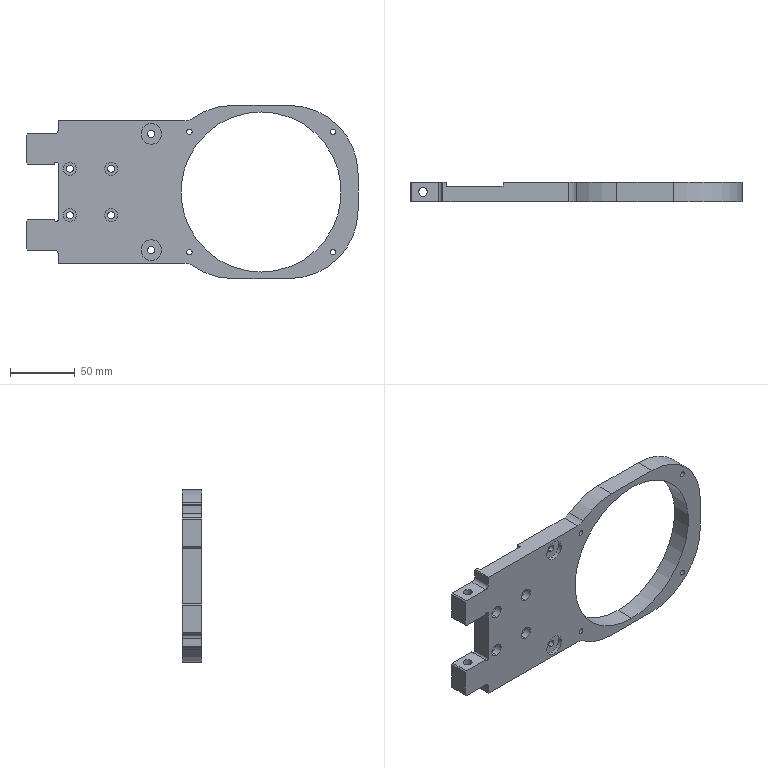Part | SolidWorks | features BaseBody 1 | 1 solid | 87 faces | box 257 x 15 x 134 mm | volume 222484 mm3 | cylinder 53 | plane 34 | commonest cylinder face diameters 5.5 x12 10 x12 4.2 x8 6.8 x4 16 x4 106 x4